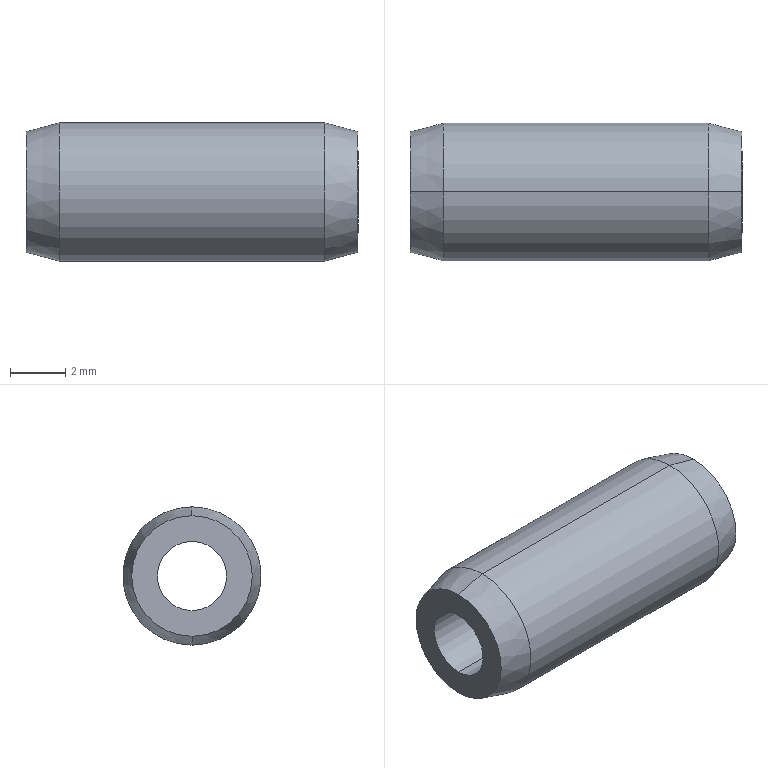Part | STEP file | GB/T 119 5×12 | 1 solid | 10 faces | box 12 x 5 x 5 mm | volume 170.914 mm3 | cylinder 4 | cone 4 | plane 2 | commonest cylinder face diameters 2.5 x2 5 x2
STEP:
#1=CARTESIAN_POINT('',(-2.2,0.,1.25));
#2=VERTEX_POINT('',#1);
#3=CARTESIAN_POINT('',(-2.2,0.,-1.25));
#4=VERTEX_POINT('',#3);
#5=CARTESIAN_POINT('',(-2.2,0.,0.));
#6=DIRECTION('',(1.,0.,0.));
#7=DIRECTION('',(0.,0.,-1.));
#8=AXIS2_PLACEMENT_3D('',#5,#6,#7);
#9=CIRCLE('',#8,1.25);
#10=EDGE_CURVE('',#2,#4,#9,.T.);
#11=ORIENTED_EDGE('',*,*,#10,.F.);
#12=CARTESIAN_POINT('',(9.8,0.,1.25));
#13=VERTEX_POINT('',#12);
#14=CARTESIAN_POINT('',(9.8,0.,1.25));
#15=DIRECTION('',(1.,0.,0.));
#16=VECTOR('',#15,1000.);
#17=LINE('',#14,#16);
#18=EDGE_CURVE('',#2,#13,#17,.T.);
#19=ORIENTED_EDGE('',*,*,#18,.T.);
#20=CARTESIAN_POINT('',(9.8,0.,-1.25));
#21=VERTEX_POINT('',#20);
#22=CARTESIAN_POINT('',(9.8,0.,0.));
#23=DIRECTION('',(1.,0.,0.));
#24=DIRECTION('',(0.,0.,-1.));
#25=AXIS2_PLACEMENT_3D('',#22,#23,#24);
#26=CIRCLE('',#25,1.25);
#27=EDGE_CURVE('',#13,#21,#26,.T.);
#28=ORIENTED_EDGE('',*,*,#27,.T.);
#29=CARTESIAN_POINT('',(9.8,0.,-1.25));
#30=DIRECTION('',(1.,0.,0.));
#31=VECTOR('',#30,1000.);
#32=LINE('',#29,#31);
#33=EDGE_CURVE('',#4,#21,#32,.T.);
#34=ORIENTED_EDGE('',*,*,#33,.F.);
#35=EDGE_LOOP('',(#11,#19,#28,#34));
#36=FACE_OUTER_BOUND('',#35,.T.);
#37=CARTESIAN_POINT('',(9.8,0.,0.));
#38=DIRECTION('',(1.,0.,0.));
#39=DIRECTION('',(0.,0.,-1.));
#40=AXIS2_PLACEMENT_3D('',#37,#38,#39);
#41=CYLINDRICAL_SURFACE('',#40,1.25);
#42=ADVANCED_FACE('',(#36),#41,.F.);
#43=CARTESIAN_POINT('',(8.6,0.,2.5));
#44=VERTEX_POINT('',#43);
#45=CARTESIAN_POINT('',(8.6,0.,-2.5));
#46=VERTEX_POINT('',#45);
#47=CARTESIAN_POINT('',(8.6,0.,0.));
#48=DIRECTION('',(-1.,0.,0.));
#49=DIRECTION('',(0.,0.,1.));
#50=AXIS2_PLACEMENT_3D('',#47,#48,#49);
#51=CIRCLE('',#50,2.5);
#52=EDGE_CURVE('',#44,#46,#51,.T.);
#53=ORIENTED_EDGE('',*,*,#52,.T.);
#54=CARTESIAN_POINT('',(-1.,0.,-2.5));
#55=VERTEX_POINT('',#54);
#56=CARTESIAN_POINT('',(0.,0.,-2.5));
#57=DIRECTION('',(-1.,0.,0.));
#58=VECTOR('',#57,1000.);
#59=LINE('',#56,#58);
#60=EDGE_CURVE('',#46,#55,#59,.T.);
#61=ORIENTED_EDGE('',*,*,#60,.T.);
#62=CARTESIAN_POINT('',(-1.,0.,2.5));
#63=VERTEX_POINT('',#62);
#64=CARTESIAN_POINT('',(-1.,0.,0.));
#65=DIRECTION('',(-1.,0.,0.));
#66=DIRECTION('',(0.,0.,1.));
#67=AXIS2_PLACEMENT_3D('',#64,#65,#66);
#68=CIRCLE('',#67,2.5);
#69=EDGE_CURVE('',#63,#55,#68,.T.);
#70=ORIENTED_EDGE('',*,*,#69,.F.);
#71=CARTESIAN_POINT('',(0.,0.,2.5));
#72=DIRECTION('',(-1.,0.,0.));
#73=VECTOR('',#72,1000.);
#74=LINE('',#71,#73);
#75=EDGE_CURVE('',#44,#63,#74,.T.);
#76=ORIENTED_EDGE('',*,*,#75,.F.);
#77=EDGE_LOOP('',(#53,#61,#70,#76));
#78=FACE_OUTER_BOUND('',#77,.T.);
#79=CARTESIAN_POINT('',(0.,0.,0.));
#80=DIRECTION('',(-1.,0.,0.));
#81=DIRECTION('',(0.,0.,1.));
#82=AXIS2_PLACEMENT_3D('',#79,#80,#81);
#83=CYLINDRICAL_SURFACE('',#82,2.5);
#84=ADVANCED_FACE('',(#78),#83,.T.);
#85=CARTESIAN_POINT('',(-2.2,0.,2.178));
#86=VERTEX_POINT('',#85);
#87=CARTESIAN_POINT('',(-2.2,0.,-2.178));
#88=VERTEX_POINT('',#87);
#89=CARTESIAN_POINT('',(-2.2,0.,0.));
#90=DIRECTION('',(-1.,0.,0.));
#91=DIRECTION('',(0.,0.,1.));
#92=AXIS2_PLACEMENT_3D('',#89,#90,#91);
#93=CIRCLE('',#92,2.178);
#94=EDGE_CURVE('',#86,#88,#93,.T.);
#95=ORIENTED_EDGE('',*,*,#94,.F.);
#96=CARTESIAN_POINT('',(-1.,0.,2.5));
#97=DIRECTION('',(0.9659,0.,0.2588));
#98=VECTOR('',#97,1000.);
#99=LINE('',#96,#98);
#100=EDGE_CURVE('',#86,#63,#99,.T.);
#101=ORIENTED_EDGE('',*,*,#100,.T.);
#102=ORIENTED_EDGE('',*,*,#69,.T.);
#103=CARTESIAN_POINT('',(-1.,0.,-2.5));
#104=DIRECTION('',(0.9659,0.,-0.2588));
#105=VECTOR('',#104,1000.);
#106=LINE('',#103,#105);
#107=EDGE_CURVE('',#88,#55,#106,.T.);
#108=ORIENTED_EDGE('',*,*,#107,.F.);
#109=EDGE_LOOP('',(#95,#101,#102,#108));
#110=FACE_OUTER_BOUND('',#109,.T.);
#111=CARTESIAN_POINT('',(-1.,0.,0.));
#112=DIRECTION('',(1.,0.,0.));
#113=DIRECTION('',(0.,0.,-1.));
#114=AXIS2_PLACEMENT_3D('',#111,#112,#113);
#115=CONICAL_SURFACE('',#114,2.5,0.2618);
#116=ADVANCED_FACE('',(#110),#115,.T.);
#117=CARTESIAN_POINT('',(9.8,0.,2.178));
#118=VERTEX_POINT('',#117);
#119=CARTESIAN_POINT('',(9.8,0.,-2.178));
#120=VERTEX_POINT('',#119);
#121=CARTESIAN_POINT('',(9.8,0.,0.));
#122=DIRECTION('',(-1.,0.,0.));
#123=DIRECTION('',(0.,0.,1.));
#124=AXIS2_PLACEMENT_3D('',#121,#122,#123);
#125=CIRCLE('',#124,2.178);
#126=EDGE_CURVE('',#118,#120,#125,.T.);
#127=ORIENTED_EDGE('',*,*,#126,.T.);
#128=CARTESIAN_POINT('',(9.8,0.,-2.178));
#129=DIRECTION('',(-0.9659,0.,-0.2588));
#130=VECTOR('',#129,1000.);
#131=LINE('',#128,#130);
#132=EDGE_CURVE('',#120,#46,#131,.T.);
#133=ORIENTED_EDGE('',*,*,#132,.T.);
#134=ORIENTED_EDGE('',*,*,#52,.F.);
#135=CARTESIAN_POINT('',(9.8,0.,2.178));
#136=DIRECTION('',(-0.9659,0.,0.2588));
#137=VECTOR('',#136,1000.);
#138=LINE('',#135,#137);
#139=EDGE_CURVE('',#118,#44,#138,.T.);
#140=ORIENTED_EDGE('',*,*,#139,.F.);
#141=EDGE_LOOP('',(#127,#133,#134,#140));
#142=FACE_OUTER_BOUND('',#141,.T.);
#143=CARTESIAN_POINT('',(9.8,0.,0.));
#144=DIRECTION('',(-1.,0.,0.));
#145=DIRECTION('',(0.,0.,1.));
#146=AXIS2_PLACEMENT_3D('',#143,#144,#145);
#147=CONICAL_SURFACE('',#146,2.178,0.2618);
#148=ADVANCED_FACE('',(#142),#147,.T.);
#149=ORIENTED_EDGE('',*,*,#132,.F.);
#150=CARTESIAN_POINT('',(9.8,0.,0.));
#151=DIRECTION('',(-1.,0.,0.));
#152=DIRECTION('',(0.,0.,1.));
#153=AXIS2_PLACEMENT_3D('',#150,#151,#152);
#154=CIRCLE('',#153,2.178);
#155=EDGE_CURVE('',#120,#118,#154,.T.);
#156=ORIENTED_EDGE('',*,*,#155,.T.);
#157=ORIENTED_EDGE('',*,*,#139,.T.);
#158=CARTESIAN_POINT('',(8.6,0.,0.));
#159=DIRECTION('',(-1.,0.,0.));
#160=DIRECTION('',(0.,0.,1.));
#161=AXIS2_PLACEMENT_3D('',#158,#159,#160);
#162=CIRCLE('',#161,2.5);
#163=EDGE_CURVE('',#46,#44,#162,.T.);
#164=ORIENTED_EDGE('',*,*,#163,.F.);
#165=EDGE_LOOP('',(#149,#156,#157,#164));
#166=FACE_OUTER_BOUND('',#165,.T.);
#167=CARTESIAN_POINT('',(9.8,0.,0.));
#168=DIRECTION('',(-1.,0.,0.));
#169=DIRECTION('',(0.,0.,1.));
#170=AXIS2_PLACEMENT_3D('',#167,#168,#169);
#171=CONICAL_SURFACE('',#170,2.178,0.2618);
#172=ADVANCED_FACE('',(#166),#171,.T.);
#173=CARTESIAN_POINT('',(9.8,0.,0.));
#174=DIRECTION('',(1.,0.,0.));
#175=DIRECTION('',(0.,0.,-1.));
#176=AXIS2_PLACEMENT_3D('',#173,#174,#175);
#177=CIRCLE('',#176,1.25);
#178=EDGE_CURVE('',#21,#13,#177,.T.);
#179=ORIENTED_EDGE('',*,*,#178,.F.);
#180=ORIENTED_EDGE('',*,*,#27,.F.);
#181=EDGE_LOOP('',(#179,#180));
#182=FACE_BOUND('',#181,.T.);
#183=ORIENTED_EDGE('',*,*,#126,.F.);
#184=ORIENTED_EDGE('',*,*,#155,.F.);
#185=EDGE_LOOP('',(#183,#184));
#186=FACE_OUTER_BOUND('',#185,.T.);
#187=CARTESIAN_POINT('',(9.8,2.178,0.));
#188=DIRECTION('',(-1.,0.,0.));
#189=DIRECTION('',(0.,0.,1.));
#190=AXIS2_PLACEMENT_3D('',#187,#188,#189);
#191=PLANE('',#190);
#192=ADVANCED_FACE('',(#182,#186),#191,.F.);
#193=CARTESIAN_POINT('',(-2.2,0.,0.));
#194=DIRECTION('',(1.,0.,0.));
#195=DIRECTION('',(0.,0.,-1.));
#196=AXIS2_PLACEMENT_3D('',#193,#194,#195);
#197=CIRCLE('',#196,1.25);
#198=EDGE_CURVE('',#4,#2,#197,.T.);
#199=ORIENTED_EDGE('',*,*,#198,.T.);
#200=ORIENTED_EDGE('',*,*,#10,.T.);
#201=EDGE_LOOP('',(#199,#200));
#202=FACE_BOUND('',#201,.T.);
#203=CARTESIAN_POINT('',(-2.2,0.,0.));
#204=DIRECTION('',(-1.,0.,0.));
#205=DIRECTION('',(0.,0.,1.));
#206=AXIS2_PLACEMENT_3D('',#203,#204,#205);
#207=CIRCLE('',#206,2.178);
#208=EDGE_CURVE('',#88,#86,#207,.T.);
#209=ORIENTED_EDGE('',*,*,#208,.T.);
#210=ORIENTED_EDGE('',*,*,#94,.T.);
#211=EDGE_LOOP('',(#209,#210));
#212=FACE_OUTER_BOUND('',#211,.T.);
#213=CARTESIAN_POINT('',(-2.2,2.178,0.));
#214=DIRECTION('',(1.,0.,0.));
#215=DIRECTION('',(0.,0.,-1.));
#216=AXIS2_PLACEMENT_3D('',#213,#214,#215);
#217=PLANE('',#216);
#218=ADVANCED_FACE('',(#202,#212),#217,.F.);
#219=ORIENTED_EDGE('',*,*,#100,.F.);
#220=ORIENTED_EDGE('',*,*,#208,.F.);
#221=ORIENTED_EDGE('',*,*,#107,.T.);
#222=CARTESIAN_POINT('',(-1.,0.,0.));
#223=DIRECTION('',(-1.,0.,0.));
#224=DIRECTION('',(0.,0.,1.));
#225=AXIS2_PLACEMENT_3D('',#222,#223,#224);
#226=CIRCLE('',#225,2.5);
#227=EDGE_CURVE('',#55,#63,#226,.T.);
#228=ORIENTED_EDGE('',*,*,#227,.T.);
#229=EDGE_LOOP('',(#219,#220,#221,#228));
#230=FACE_OUTER_BOUND('',#229,.T.);
#231=CARTESIAN_POINT('',(-1.,0.,0.));
#232=DIRECTION('',(1.,0.,0.));
#233=DIRECTION('',(0.,0.,-1.));
#234=AXIS2_PLACEMENT_3D('',#231,#232,#233);
#235=CONICAL_SURFACE('',#234,2.5,0.2618);
#236=ADVANCED_FACE('',(#230),#235,.T.);
#237=ORIENTED_EDGE('',*,*,#60,.F.);
#238=ORIENTED_EDGE('',*,*,#163,.T.);
#239=ORIENTED_EDGE('',*,*,#75,.T.);
#240=ORIENTED_EDGE('',*,*,#227,.F.);
#241=EDGE_LOOP('',(#237,#238,#239,#240));
#242=FACE_OUTER_BOUND('',#241,.T.);
#243=CARTESIAN_POINT('',(0.,0.,0.));
#244=DIRECTION('',(-1.,0.,0.));
#245=DIRECTION('',(0.,0.,1.));
#246=AXIS2_PLACEMENT_3D('',#243,#244,#245);
#247=CYLINDRICAL_SURFACE('',#246,2.5);
#248=ADVANCED_FACE('',(#242),#247,.T.);
#249=ORIENTED_EDGE('',*,*,#18,.F.);
#250=ORIENTED_EDGE('',*,*,#198,.F.);
#251=ORIENTED_EDGE('',*,*,#33,.T.);
#252=ORIENTED_EDGE('',*,*,#178,.T.);
#253=EDGE_LOOP('',(#249,#250,#251,#252));
#254=FACE_OUTER_BOUND('',#253,.T.);
#255=CARTESIAN_POINT('',(9.8,0.,0.));
#256=DIRECTION('',(1.,0.,0.));
#257=DIRECTION('',(0.,0.,-1.));
#258=AXIS2_PLACEMENT_3D('',#255,#256,#257);
#259=CYLINDRICAL_SURFACE('',#258,1.25);
#260=ADVANCED_FACE('',(#254),#259,.F.);
#261=CLOSED_SHELL('',(#42,#84,#116,#148,#172,#192,#218,#236,#248,#260));
#262=MANIFOLD_SOLID_BREP('',#261);
#263=CARTESIAN_POINT('',(0.,0.,0.));
#264=DIRECTION('',(0.,0.,1.));
#265=DIRECTION('',(1.,0.,0.));
#266=AXIS2_PLACEMENT_3D('',#263,#264,#265);
#267=(LENGTH_UNIT()NAMED_UNIT(*)SI_UNIT(.MILLI.,.METRE.));
#268=UNCERTAINTY_MEASURE_WITH_UNIT(LENGTH_MEASURE(0.00001),#267,'','');
#269=(NAMED_UNIT(*)PLANE_ANGLE_UNIT()SI_UNIT($,.RADIAN.));
#270=(NAMED_UNIT(*)SI_UNIT($,.STERADIAN.)SOLID_ANGLE_UNIT());
#271=(GEOMETRIC_REPRESENTATION_CONTEXT(3)GLOBAL_UNCERTAINTY_ASSIGNED_CONTEXT((#268))GLOBAL_UNIT_ASSIGNED_CONTEXT((#267,#269,#270))REPRESENTATION_CONTEXT('',''));
#272=ADVANCED_BREP_SHAPE_REPRESENTATION('',(#262,#266),#271);